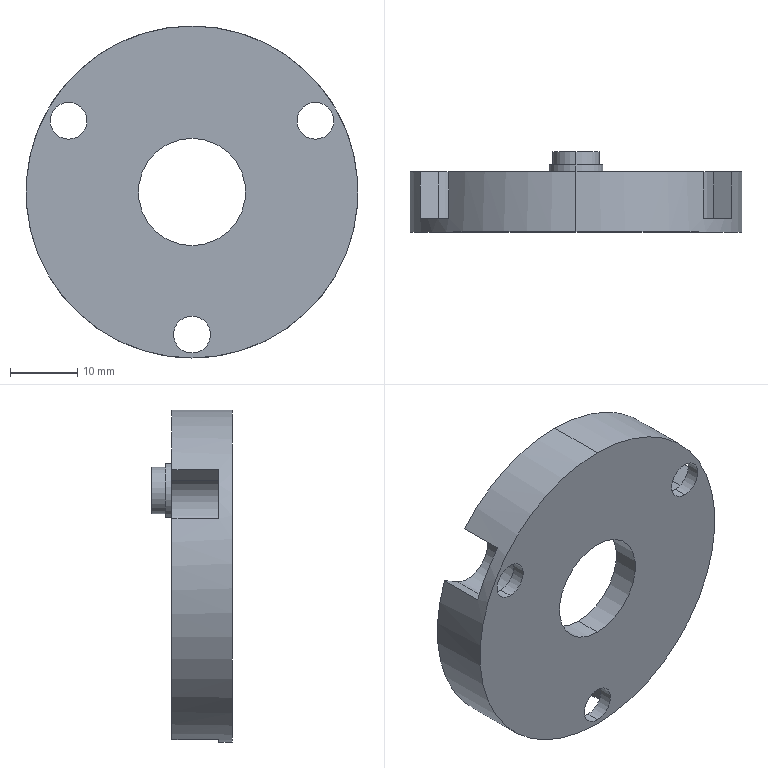Part | SolidWorks | features ICE 6, CirPattern 1, Extrusion 1, HoleWzd 1 | 1 solid | 44 faces | box 49.5 x 12 x 49.5 mm | volume 11403 mm3 | cylinder 26 | plane 14 | cone 4 | commonest cylinder face diameters 5.5 x6 4 x4 8.5 x4 5 x2 7 x2 8 x2
STEP:
#1=CARTESIAN_POINT('',(0.,4.,-8.));
#2=VERTEX_POINT('',#1);
#3=CARTESIAN_POINT('',(0.,4.,8.));
#4=VERTEX_POINT('',#3);
#5=CARTESIAN_POINT('',(0.,4.,0.));
#6=DIRECTION('',(0.,1.,0.));
#7=DIRECTION('',(0.,0.,1.));
#8=AXIS2_PLACEMENT_3D('',#5,#6,#7);
#9=CIRCLE('',#8,8.);
#10=EDGE_CURVE('',#2,#4,#9,.T.);
#11=ORIENTED_EDGE('',*,*,#10,.T.);
#12=CARTESIAN_POINT('',(0.,0.,8.));
#13=VERTEX_POINT('',#12);
#14=CARTESIAN_POINT('',(0.,5.,8.));
#15=DIRECTION('',(0.,-1.,0.));
#16=VECTOR('',#15,1000.);
#17=LINE('',#14,#16);
#18=EDGE_CURVE('',#4,#13,#17,.T.);
#19=ORIENTED_EDGE('',*,*,#18,.T.);
#20=CARTESIAN_POINT('',(0.,0.,-8.));
#21=VERTEX_POINT('',#20);
#22=CARTESIAN_POINT('',(0.,0.,0.));
#23=DIRECTION('',(0.,-1.,0.));
#24=DIRECTION('',(0.,0.,-1.));
#25=AXIS2_PLACEMENT_3D('',#22,#23,#24);
#26=CIRCLE('',#25,8.);
#27=EDGE_CURVE('',#13,#21,#26,.T.);
#28=ORIENTED_EDGE('',*,*,#27,.T.);
#29=CARTESIAN_POINT('',(0.,5.,-8.));
#30=DIRECTION('',(0.,-1.,0.));
#31=VECTOR('',#30,1000.);
#32=LINE('',#29,#31);
#33=EDGE_CURVE('',#2,#21,#32,.T.);
#34=ORIENTED_EDGE('',*,*,#33,.F.);
#35=EDGE_LOOP('',(#11,#19,#28,#34));
#36=FACE_OUTER_BOUND('',#35,.T.);
#37=CARTESIAN_POINT('',(0.,5.,0.));
#38=DIRECTION('',(0.,-1.,0.));
#39=DIRECTION('',(0.,0.,-1.));
#40=AXIS2_PLACEMENT_3D('',#37,#38,#39);
#41=CYLINDRICAL_SURFACE('',#40,8.);
#42=ADVANCED_FACE('',(#36),#41,.F.);
#43=CARTESIAN_POINT('',(9.28,4.,13.142));
#44=VERTEX_POINT('',#43);
#45=CARTESIAN_POINT('',(10.56,4.,12.678));
#46=VERTEX_POINT('',#45);
#47=CARTESIAN_POINT('',(9.28,4.,11.142));
#48=DIRECTION('',(0.,1.,0.));
#49=DIRECTION('',(0.,0.,1.));
#50=AXIS2_PLACEMENT_3D('',#47,#48,#49);
#51=CIRCLE('',#50,2.);
#52=EDGE_CURVE('',#44,#46,#51,.T.);
#53=ORIENTED_EDGE('',*,*,#52,.F.);
#54=CARTESIAN_POINT('',(9.28,9.,13.142));
#55=VERTEX_POINT('',#54);
#56=CARTESIAN_POINT('',(9.28,4.,13.142));
#57=DIRECTION('',(0.,1.,0.));
#58=VECTOR('',#57,1000.);
#59=LINE('',#56,#58);
#60=EDGE_CURVE('',#44,#55,#59,.T.);
#61=ORIENTED_EDGE('',*,*,#60,.T.);
#62=CARTESIAN_POINT('',(10.56,9.,12.678));
#63=VERTEX_POINT('',#62);
#64=CARTESIAN_POINT('',(9.28,9.,11.142));
#65=DIRECTION('',(0.,1.,0.));
#66=DIRECTION('',(0.,0.,1.));
#67=AXIS2_PLACEMENT_3D('',#64,#65,#66);
#68=CIRCLE('',#67,2.);
#69=EDGE_CURVE('',#55,#63,#68,.T.);
#70=ORIENTED_EDGE('',*,*,#69,.T.);
#71=CARTESIAN_POINT('',(10.56,4.,12.678));
#72=DIRECTION('',(0.,1.,0.));
#73=VECTOR('',#72,1000.);
#74=LINE('',#71,#73);
#75=EDGE_CURVE('',#46,#63,#74,.T.);
#76=ORIENTED_EDGE('',*,*,#75,.F.);
#77=EDGE_LOOP('',(#53,#61,#70,#76));
#78=FACE_OUTER_BOUND('',#77,.T.);
#79=CARTESIAN_POINT('',(9.28,4.,11.142));
#80=DIRECTION('',(0.,1.,0.));
#81=DIRECTION('',(0.,0.,1.));
#82=AXIS2_PLACEMENT_3D('',#79,#80,#81);
#83=CYLINDRICAL_SURFACE('',#82,2.);
#84=ADVANCED_FACE('',(#78),#83,.F.);
#85=CARTESIAN_POINT('',(-9.28,4.,13.142));
#86=VERTEX_POINT('',#85);
#87=CARTESIAN_POINT('',(-7.733,4.,12.41));
#88=VERTEX_POINT('',#87);
#89=CARTESIAN_POINT('',(-9.28,4.,11.142));
#90=DIRECTION('',(0.,1.,0.));
#91=DIRECTION('',(0.,0.,1.));
#92=AXIS2_PLACEMENT_3D('',#89,#90,#91);
#93=CIRCLE('',#92,2.);
#94=EDGE_CURVE('',#86,#88,#93,.T.);
#95=ORIENTED_EDGE('',*,*,#94,.F.);
#96=CARTESIAN_POINT('',(-9.28,9.,13.142));
#97=VERTEX_POINT('',#96);
#98=CARTESIAN_POINT('',(-9.28,4.,13.142));
#99=DIRECTION('',(0.,1.,0.));
#100=VECTOR('',#99,1000.);
#101=LINE('',#98,#100);
#102=EDGE_CURVE('',#86,#97,#101,.T.);
#103=ORIENTED_EDGE('',*,*,#102,.T.);
#104=CARTESIAN_POINT('',(-7.733,9.,12.41));
#105=VERTEX_POINT('',#104);
#106=CARTESIAN_POINT('',(-9.28,9.,11.142));
#107=DIRECTION('',(0.,1.,0.));
#108=DIRECTION('',(0.,0.,1.));
#109=AXIS2_PLACEMENT_3D('',#106,#107,#108);
#110=CIRCLE('',#109,2.);
#111=EDGE_CURVE('',#97,#105,#110,.T.);
#112=ORIENTED_EDGE('',*,*,#111,.T.);
#113=CARTESIAN_POINT('',(-7.733,4.,12.41));
#114=DIRECTION('',(0.,1.,0.));
#115=VECTOR('',#114,1000.);
#116=LINE('',#113,#115);
#117=EDGE_CURVE('',#88,#105,#116,.T.);
#118=ORIENTED_EDGE('',*,*,#117,.F.);
#119=EDGE_LOOP('',(#95,#103,#112,#118));
#120=FACE_OUTER_BOUND('',#119,.T.);
#121=CARTESIAN_POINT('',(-9.28,4.,11.142));
#122=DIRECTION('',(0.,1.,0.));
#123=DIRECTION('',(0.,0.,1.));
#124=AXIS2_PLACEMENT_3D('',#121,#122,#123);
#125=CYLINDRICAL_SURFACE('',#124,2.);
#126=ADVANCED_FACE('',(#120),#125,.F.);
#127=CARTESIAN_POINT('',(0.,11.975,10.25));
#128=VERTEX_POINT('',#127);
#129=CARTESIAN_POINT('',(0.,11.975,15.25));
#130=VERTEX_POINT('',#129);
#131=CARTESIAN_POINT('',(0.,11.975,12.75));
#132=DIRECTION('',(0.,1.,0.));
#133=DIRECTION('',(0.,0.,1.));
#134=AXIS2_PLACEMENT_3D('',#131,#132,#133);
#135=CIRCLE('',#134,2.5);
#136=EDGE_CURVE('',#128,#130,#135,.T.);
#137=ORIENTED_EDGE('',*,*,#136,.F.);
#138=CARTESIAN_POINT('',(0.,12.,10.225));
#139=VERTEX_POINT('',#138);
#140=CARTESIAN_POINT('',(0.,12.,10.225));
#141=DIRECTION('',(0.,0.7071,-0.7071));
#142=VECTOR('',#141,1000.);
#143=LINE('',#140,#142);
#144=EDGE_CURVE('',#128,#139,#143,.T.);
#145=ORIENTED_EDGE('',*,*,#144,.T.);
#146=CARTESIAN_POINT('',(0.,12.,15.275));
#147=VERTEX_POINT('',#146);
#148=CARTESIAN_POINT('',(0.,12.,12.75));
#149=DIRECTION('',(0.,1.,0.));
#150=DIRECTION('',(0.,0.,1.));
#151=AXIS2_PLACEMENT_3D('',#148,#149,#150);
#152=CIRCLE('',#151,2.525);
#153=EDGE_CURVE('',#139,#147,#152,.T.);
#154=ORIENTED_EDGE('',*,*,#153,.T.);
#155=CARTESIAN_POINT('',(0.,12.,15.275));
#156=DIRECTION('',(0.,0.7071,0.7071));
#157=VECTOR('',#156,1000.);
#158=LINE('',#155,#157);
#159=EDGE_CURVE('',#130,#147,#158,.T.);
#160=ORIENTED_EDGE('',*,*,#159,.F.);
#161=EDGE_LOOP('',(#137,#145,#154,#160));
#162=FACE_OUTER_BOUND('',#161,.T.);
#163=CARTESIAN_POINT('',(0.,12.,12.75));
#164=DIRECTION('',(0.,1.,0.));
#165=DIRECTION('',(0.,0.,1.));
#166=AXIS2_PLACEMENT_3D('',#163,#164,#165);
#167=CONICAL_SURFACE('',#166,2.525,0.7854);
#168=ADVANCED_FACE('',(#162),#167,.F.);
#169=CARTESIAN_POINT('',(0.,7.,10.25));
#170=VERTEX_POINT('',#169);
#171=CARTESIAN_POINT('',(0.,7.,15.25));
#172=VERTEX_POINT('',#171);
#173=CARTESIAN_POINT('',(0.,7.,12.75));
#174=DIRECTION('',(0.,1.,0.));
#175=DIRECTION('',(0.,0.,1.));
#176=AXIS2_PLACEMENT_3D('',#173,#174,#175);
#177=CIRCLE('',#176,2.5);
#178=EDGE_CURVE('',#170,#172,#177,.T.);
#179=ORIENTED_EDGE('',*,*,#178,.F.);
#180=CARTESIAN_POINT('',(0.,12.,10.25));
#181=DIRECTION('',(0.,1.,0.));
#182=VECTOR('',#181,1000.);
#183=LINE('',#180,#182);
#184=EDGE_CURVE('',#170,#128,#183,.T.);
#185=ORIENTED_EDGE('',*,*,#184,.T.);
#186=ORIENTED_EDGE('',*,*,#136,.T.);
#187=CARTESIAN_POINT('',(0.,12.,15.25));
#188=DIRECTION('',(0.,1.,0.));
#189=VECTOR('',#188,1000.);
#190=LINE('',#187,#189);
#191=EDGE_CURVE('',#172,#130,#190,.T.);
#192=ORIENTED_EDGE('',*,*,#191,.F.);
#193=EDGE_LOOP('',(#179,#185,#186,#192));
#194=FACE_OUTER_BOUND('',#193,.T.);
#195=CARTESIAN_POINT('',(0.,12.,12.75));
#196=DIRECTION('',(0.,1.,0.));
#197=DIRECTION('',(0.,0.,1.));
#198=AXIS2_PLACEMENT_3D('',#195,#196,#197);
#199=CYLINDRICAL_SURFACE('',#198,2.5);
#200=ADVANCED_FACE('',(#194),#199,.F.);
#201=CARTESIAN_POINT('',(0.,5.498,12.75));
#202=VERTEX_POINT('',#201);
#203=CARTESIAN_POINT('',(0.,7.,15.25));
#204=DIRECTION('',(0.,0.515,0.8572));
#205=VECTOR('',#204,1000.);
#206=LINE('',#203,#205);
#207=EDGE_CURVE('',#202,#172,#206,.T.);
#208=ORIENTED_EDGE('',*,*,#207,.F.);
#209=CARTESIAN_POINT('',(0.,7.,10.25));
#210=DIRECTION('',(0.,0.515,-0.8572));
#211=VECTOR('',#210,1000.);
#212=LINE('',#209,#211);
#213=EDGE_CURVE('',#202,#170,#212,.T.);
#214=ORIENTED_EDGE('',*,*,#213,.T.);
#215=ORIENTED_EDGE('',*,*,#178,.T.);
#216=EDGE_LOOP('',(#208,#214,#215));
#217=FACE_OUTER_BOUND('',#216,.T.);
#218=CARTESIAN_POINT('',(0.,7.,12.75));
#219=DIRECTION('',(0.,1.,0.));
#220=DIRECTION('',(0.,0.,1.));
#221=AXIS2_PLACEMENT_3D('',#218,#219,#220);
#222=CONICAL_SURFACE('',#221,2.5,1.03);
#223=ADVANCED_FACE('',(#217),#222,.F.);
#224=CARTESIAN_POINT('',(0.,12.,16.25));
#225=VERTEX_POINT('',#224);
#226=CARTESIAN_POINT('',(0.,12.,9.25));
#227=VERTEX_POINT('',#226);
#228=CARTESIAN_POINT('',(0.,12.,12.75));
#229=DIRECTION('',(0.,1.,0.));
#230=DIRECTION('',(0.,0.,1.));
#231=AXIS2_PLACEMENT_3D('',#228,#229,#230);
#232=CIRCLE('',#231,3.5);
#233=EDGE_CURVE('',#225,#227,#232,.T.);
#234=ORIENTED_EDGE('',*,*,#233,.F.);
#235=CARTESIAN_POINT('',(0.,10.,16.25));
#236=VERTEX_POINT('',#235);
#237=CARTESIAN_POINT('',(0.,12.,16.25));
#238=DIRECTION('',(0.,-1.,0.));
#239=VECTOR('',#238,1000.);
#240=LINE('',#237,#239);
#241=EDGE_CURVE('',#225,#236,#240,.T.);
#242=ORIENTED_EDGE('',*,*,#241,.T.);
#243=CARTESIAN_POINT('',(0.,10.,9.25));
#244=VERTEX_POINT('',#243);
#245=CARTESIAN_POINT('',(0.,10.,12.75));
#246=DIRECTION('',(0.,-1.,0.));
#247=DIRECTION('',(0.,0.,1.));
#248=AXIS2_PLACEMENT_3D('',#245,#246,#247);
#249=CIRCLE('',#248,3.5);
#250=EDGE_CURVE('',#244,#236,#249,.T.);
#251=ORIENTED_EDGE('',*,*,#250,.F.);
#252=CARTESIAN_POINT('',(0.,12.,9.25));
#253=DIRECTION('',(0.,-1.,0.));
#254=VECTOR('',#253,1000.);
#255=LINE('',#252,#254);
#256=EDGE_CURVE('',#227,#244,#255,.T.);
#257=ORIENTED_EDGE('',*,*,#256,.F.);
#258=EDGE_LOOP('',(#234,#242,#251,#257));
#259=FACE_OUTER_BOUND('',#258,.T.);
#260=CARTESIAN_POINT('',(0.,12.,12.75));
#261=DIRECTION('',(0.,-1.,0.));
#262=DIRECTION('',(0.,0.,-1.));
#263=AXIS2_PLACEMENT_3D('',#260,#261,#262);
#264=CYLINDRICAL_SURFACE('',#263,3.5);
#265=ADVANCED_FACE('',(#259),#264,.T.);
#266=CARTESIAN_POINT('',(0.,10.,16.75));
#267=VERTEX_POINT('',#266);
#268=CARTESIAN_POINT('',(0.,10.,8.75));
#269=VERTEX_POINT('',#268);
#270=CARTESIAN_POINT('',(0.,10.,12.75));
#271=DIRECTION('',(0.,1.,0.));
#272=DIRECTION('',(0.,0.,1.));
#273=AXIS2_PLACEMENT_3D('',#270,#271,#272);
#274=CIRCLE('',#273,4.);
#275=EDGE_CURVE('',#267,#269,#274,.T.);
#276=ORIENTED_EDGE('',*,*,#275,.F.);
#277=CARTESIAN_POINT('',(0.,9.,16.75));
#278=VERTEX_POINT('',#277);
#279=CARTESIAN_POINT('',(0.,10.,16.75));
#280=DIRECTION('',(0.,-1.,0.));
#281=VECTOR('',#280,1000.);
#282=LINE('',#279,#281);
#283=EDGE_CURVE('',#267,#278,#282,.T.);
#284=ORIENTED_EDGE('',*,*,#283,.T.);
#285=CARTESIAN_POINT('',(0.,9.,8.75));
#286=VERTEX_POINT('',#285);
#287=CARTESIAN_POINT('',(0.,9.,12.75));
#288=DIRECTION('',(0.,1.,0.));
#289=DIRECTION('',(0.,0.,1.));
#290=AXIS2_PLACEMENT_3D('',#287,#288,#289);
#291=CIRCLE('',#290,4.);
#292=EDGE_CURVE('',#278,#286,#291,.T.);
#293=ORIENTED_EDGE('',*,*,#292,.T.);
#294=CARTESIAN_POINT('',(0.,10.,8.75));
#295=DIRECTION('',(0.,-1.,0.));
#296=VECTOR('',#295,1000.);
#297=LINE('',#294,#296);
#298=EDGE_CURVE('',#269,#286,#297,.T.);
#299=ORIENTED_EDGE('',*,*,#298,.F.);
#300=EDGE_LOOP('',(#276,#284,#293,#299));
#301=FACE_OUTER_BOUND('',#300,.T.);
#302=CARTESIAN_POINT('',(0.,10.,12.75));
#303=DIRECTION('',(0.,-1.,0.));
#304=DIRECTION('',(0.,0.,-1.));
#305=AXIS2_PLACEMENT_3D('',#302,#303,#304);
#306=CYLINDRICAL_SURFACE('',#305,4.);
#307=ADVANCED_FACE('',(#301),#306,.T.);
#308=CARTESIAN_POINT('',(18.403,0.,7.875));
#309=VERTEX_POINT('',#308);
#310=CARTESIAN_POINT('',(18.403,0.,13.375));
#311=VERTEX_POINT('',#310);
#312=CARTESIAN_POINT('',(18.403,0.,10.625));
#313=DIRECTION('',(0.,1.,0.));
#314=DIRECTION('',(0.,0.,1.));
#315=AXIS2_PLACEMENT_3D('',#312,#313,#314);
#316=CIRCLE('',#315,2.75);
#317=EDGE_CURVE('',#309,#311,#316,.T.);
#318=ORIENTED_EDGE('',*,*,#317,.F.);
#319=CARTESIAN_POINT('',(18.403,2.,7.875));
#320=VERTEX_POINT('',#319);
#321=CARTESIAN_POINT('',(18.403,-5.,7.875));
#322=DIRECTION('',(0.,1.,0.));
#323=VECTOR('',#322,1000.);
#324=LINE('',#321,#323);
#325=EDGE_CURVE('',#309,#320,#324,.T.);
#326=ORIENTED_EDGE('',*,*,#325,.T.);
#327=CARTESIAN_POINT('',(18.403,2.,13.375));
#328=VERTEX_POINT('',#327);
#329=CARTESIAN_POINT('',(18.403,2.,10.625));
#330=DIRECTION('',(0.,1.,0.));
#331=DIRECTION('',(-0.866,0.,-0.5));
#332=AXIS2_PLACEMENT_3D('',#329,#330,#331);
#333=CIRCLE('',#332,2.75);
#334=EDGE_CURVE('',#320,#328,#333,.T.);
#335=ORIENTED_EDGE('',*,*,#334,.T.);
#336=CARTESIAN_POINT('',(18.403,-5.,13.375));
#337=DIRECTION('',(0.,1.,0.));
#338=VECTOR('',#337,1000.);
#339=LINE('',#336,#338);
#340=EDGE_CURVE('',#311,#328,#339,.T.);
#341=ORIENTED_EDGE('',*,*,#340,.F.);
#342=EDGE_LOOP('',(#318,#326,#335,#341));
#343=FACE_OUTER_BOUND('',#342,.T.);
#344=CARTESIAN_POINT('',(18.403,-5.,10.625));
#345=DIRECTION('',(0.,1.,0.));
#346=DIRECTION('',(0.,0.,1.));
#347=AXIS2_PLACEMENT_3D('',#344,#345,#346);
#348=CYLINDRICAL_SURFACE('',#347,2.75);
#349=ADVANCED_FACE('',(#343),#348,.F.);
#350=CARTESIAN_POINT('',(-18.403,0.,7.875));
#351=VERTEX_POINT('',#350);
#352=CARTESIAN_POINT('',(-18.403,0.,13.375));
#353=VERTEX_POINT('',#352);
#354=CARTESIAN_POINT('',(-18.403,0.,10.625));
#355=DIRECTION('',(0.,1.,0.));
#356=DIRECTION('',(0.,0.,1.));
#357=AXIS2_PLACEMENT_3D('',#354,#355,#356);
#358=CIRCLE('',#357,2.75);
#359=EDGE_CURVE('',#351,#353,#358,.T.);
#360=ORIENTED_EDGE('',*,*,#359,.F.);
#361=CARTESIAN_POINT('',(-18.403,2.,7.875));
#362=VERTEX_POINT('',#361);
#363=CARTESIAN_POINT('',(-18.403,-5.,7.875));
#364=DIRECTION('',(0.,1.,0.));
#365=VECTOR('',#364,1000.);
#366=LINE('',#363,#365);
#367=EDGE_CURVE('',#351,#362,#366,.T.);
#368=ORIENTED_EDGE('',*,*,#367,.T.);
#369=CARTESIAN_POINT('',(-18.403,2.,13.375));
#370=VERTEX_POINT('',#369);
#371=CARTESIAN_POINT('',(-18.403,2.,10.625));
#372=DIRECTION('',(0.,1.,0.));
#373=DIRECTION('',(0.866,0.,-0.5));
#374=AXIS2_PLACEMENT_3D('',#371,#372,#373);
#375=CIRCLE('',#374,2.75);
#376=EDGE_CURVE('',#362,#370,#375,.T.);
#377=ORIENTED_EDGE('',*,*,#376,.T.);
#378=CARTESIAN_POINT('',(-18.403,-5.,13.375));
#379=DIRECTION('',(0.,1.,0.));
#380=VECTOR('',#379,1000.);
#381=LINE('',#378,#380);
#382=EDGE_CURVE('',#353,#370,#381,.T.);
#383=ORIENTED_EDGE('',*,*,#382,.F.);
#384=EDGE_LOOP('',(#360,#368,#377,#383));
#385=FACE_OUTER_BOUND('',#384,.T.);
#386=CARTESIAN_POINT('',(-18.403,-5.,10.625));
#387=DIRECTION('',(0.,1.,0.));
#388=DIRECTION('',(0.,0.,1.));
#389=AXIS2_PLACEMENT_3D('',#386,#387,#388);
#390=CYLINDRICAL_SURFACE('',#389,2.75);
#391=ADVANCED_FACE('',(#385),#390,.F.);
#392=CARTESIAN_POINT('',(0.,0.,-24.));
#393=VERTEX_POINT('',#392);
#394=CARTESIAN_POINT('',(0.,0.,-18.5));
#395=VERTEX_POINT('',#394);
#396=CARTESIAN_POINT('',(0.,0.,-21.25));
#397=DIRECTION('',(0.,1.,0.));
#398=DIRECTION('',(0.,0.,1.));
#399=AXIS2_PLACEMENT_3D('',#396,#397,#398);
#400=CIRCLE('',#399,2.75);
#401=EDGE_CURVE('',#393,#395,#400,.T.);
#402=ORIENTED_EDGE('',*,*,#401,.F.);
#403=CARTESIAN_POINT('',(0.,2.,-24.));
#404=VERTEX_POINT('',#403);
#405=CARTESIAN_POINT('',(0.,-5.,-24.));
#406=DIRECTION('',(0.,1.,0.));
#407=VECTOR('',#406,1000.);
#408=LINE('',#405,#407);
#409=EDGE_CURVE('',#393,#404,#408,.T.);
#410=ORIENTED_EDGE('',*,*,#409,.T.);
#411=CARTESIAN_POINT('',(0.,2.,-18.5));
#412=VERTEX_POINT('',#411);
#413=CARTESIAN_POINT('',(0.,2.,-21.25));
#414=DIRECTION('',(0.,1.,0.));
#415=DIRECTION('',(0.,0.,1.));
#416=AXIS2_PLACEMENT_3D('',#413,#414,#415);
#417=CIRCLE('',#416,2.75);
#418=EDGE_CURVE('',#404,#412,#417,.T.);
#419=ORIENTED_EDGE('',*,*,#418,.T.);
#420=CARTESIAN_POINT('',(0.,-5.,-18.5));
#421=DIRECTION('',(0.,1.,0.));
#422=VECTOR('',#421,1000.);
#423=LINE('',#420,#422);
#424=EDGE_CURVE('',#395,#412,#423,.T.);
#425=ORIENTED_EDGE('',*,*,#424,.F.);
#426=EDGE_LOOP('',(#402,#410,#419,#425));
#427=FACE_OUTER_BOUND('',#426,.T.);
#428=CARTESIAN_POINT('',(0.,-5.,-21.25));
#429=DIRECTION('',(0.,1.,0.));
#430=DIRECTION('',(0.,0.,1.));
#431=AXIS2_PLACEMENT_3D('',#428,#429,#430);
#432=CYLINDRICAL_SURFACE('',#431,2.75);
#433=ADVANCED_FACE('',(#427),#432,.F.);
#434=CARTESIAN_POINT('',(0.,2.,-17.));
#435=VERTEX_POINT('',#434);
#436=CARTESIAN_POINT('',(4.25,2.,-21.25));
#437=VERTEX_POINT('',#436);
#438=CARTESIAN_POINT('',(0.,2.,-21.25));
#439=DIRECTION('',(0.,1.,0.));
#440=DIRECTION('',(0.,0.,1.));
#441=AXIS2_PLACEMENT_3D('',#438,#439,#440);
#442=CIRCLE('',#441,4.25);
#443=EDGE_CURVE('',#435,#437,#442,.T.);
#444=ORIENTED_EDGE('',*,*,#443,.F.);
#445=CARTESIAN_POINT('',(0.,9.,-17.));
#446=VERTEX_POINT('',#445);
#447=CARTESIAN_POINT('',(0.,2.,-17.));
#448=DIRECTION('',(0.,1.,0.));
#449=VECTOR('',#448,1000.);
#450=LINE('',#447,#449);
#451=EDGE_CURVE('',#435,#446,#450,.T.);
#452=ORIENTED_EDGE('',*,*,#451,.T.);
#453=CARTESIAN_POINT('',(4.25,9.,-21.25));
#454=VERTEX_POINT('',#453);
#455=CARTESIAN_POINT('',(0.,9.,-21.25));
#456=DIRECTION('',(0.,1.,0.));
#457=DIRECTION('',(0.,0.,1.));
#458=AXIS2_PLACEMENT_3D('',#455,#456,#457);
#459=CIRCLE('',#458,4.25);
#460=EDGE_CURVE('',#446,#454,#459,.T.);
#461=ORIENTED_EDGE('',*,*,#460,.T.);
#462=CARTESIAN_POINT('',(4.25,2.,-21.25));
#463=DIRECTION('',(0.,1.,0.));
#464=VECTOR('',#463,1000.);
#465=LINE('',#462,#464);
#466=EDGE_CURVE('',#437,#454,#465,.T.);
#467=ORIENTED_EDGE('',*,*,#466,.F.);
#468=EDGE_LOOP('',(#444,#452,#461,#467));
#469=FACE_OUTER_BOUND('',#468,.T.);
#470=CARTESIAN_POINT('',(0.,2.,-21.25));
#471=DIRECTION('',(0.,1.,0.));
#472=DIRECTION('',(0.,0.,1.));
#473=AXIS2_PLACEMENT_3D('',#470,#471,#472);
#474=CYLINDRICAL_SURFACE('',#473,4.25);
#475=ADVANCED_FACE('',(#469),#474,.F.);
#476=CARTESIAN_POINT('',(0.,9.,24.75));
#477=VERTEX_POINT('',#476);
#478=CARTESIAN_POINT('',(18.991,9.,15.872));
#479=VERTEX_POINT('',#478);
#480=CARTESIAN_POINT('',(0.,9.,0.));
#481=DIRECTION('',(0.,1.,0.));
#482=DIRECTION('',(0.,0.,1.));
#483=AXIS2_PLACEMENT_3D('',#480,#481,#482);
#484=CIRCLE('',#483,24.75);
#485=EDGE_CURVE('',#477,#479,#484,.T.);
#486=ORIENTED_EDGE('',*,*,#485,.F.);
#487=CARTESIAN_POINT('',(0.,0.,24.75));
#488=VERTEX_POINT('',#487);
#489=CARTESIAN_POINT('',(0.,9.,24.75));
#490=DIRECTION('',(0.,-1.,0.));
#491=VECTOR('',#490,1000.);
#492=LINE('',#489,#491);
#493=EDGE_CURVE('',#477,#488,#492,.T.);
#494=ORIENTED_EDGE('',*,*,#493,.T.);
#495=CARTESIAN_POINT('',(0.,0.,-24.75));
#496=VERTEX_POINT('',#495);
#497=CARTESIAN_POINT('',(0.,0.,0.));
#498=DIRECTION('',(0.,1.,0.));
#499=DIRECTION('',(0.,0.,1.));
#500=AXIS2_PLACEMENT_3D('',#497,#498,#499);
#501=CIRCLE('',#500,24.75);
#502=EDGE_CURVE('',#488,#496,#501,.T.);
#503=ORIENTED_EDGE('',*,*,#502,.T.);
#504=CARTESIAN_POINT('',(0.,2.,-24.75));
#505=VERTEX_POINT('',#504);
#506=CARTESIAN_POINT('',(0.,9.,-24.75));
#507=DIRECTION('',(0.,-1.,0.));
#508=VECTOR('',#507,1000.);
#509=LINE('',#506,#508);
#510=EDGE_CURVE('',#505,#496,#509,.T.);
#511=ORIENTED_EDGE('',*,*,#510,.F.);
#512=CARTESIAN_POINT('',(4.25,2.,-24.382));
#513=VERTEX_POINT('',#512);
#514=CARTESIAN_POINT('',(0.,2.,0.));
#515=DIRECTION('',(0.,1.,0.));
#516=DIRECTION('',(0.,0.,1.));
#517=AXIS2_PLACEMENT_3D('',#514,#515,#516);
#518=CIRCLE('',#517,24.75);
#519=EDGE_CURVE('',#513,#505,#518,.T.);
#520=ORIENTED_EDGE('',*,*,#519,.F.);
#521=CARTESIAN_POINT('',(4.25,9.,-24.382));
#522=VERTEX_POINT('',#521);
#523=CARTESIAN_POINT('',(4.25,9.,-24.382));
#524=DIRECTION('',(0.,-1.,0.));
#525=VECTOR('',#524,1000.);
#526=LINE('',#523,#525);
#527=EDGE_CURVE('',#522,#513,#526,.T.);
#528=ORIENTED_EDGE('',*,*,#527,.F.);
#529=CARTESIAN_POINT('',(23.241,9.,8.511));
#530=VERTEX_POINT('',#529);
#531=CARTESIAN_POINT('',(0.,9.,0.));
#532=DIRECTION('',(0.,1.,0.));
#533=DIRECTION('',(0.,0.,1.));
#534=AXIS2_PLACEMENT_3D('',#531,#532,#533);
#535=CIRCLE('',#534,24.75);
#536=EDGE_CURVE('',#530,#522,#535,.T.);
#537=ORIENTED_EDGE('',*,*,#536,.F.);
#538=CARTESIAN_POINT('',(23.241,2.,8.511));
#539=VERTEX_POINT('',#538);
#540=CARTESIAN_POINT('',(23.241,9.,8.511));
#541=DIRECTION('',(0.,1.,0.));
#542=VECTOR('',#541,1000.);
#543=LINE('',#540,#542);
#544=EDGE_CURVE('',#539,#530,#543,.T.);
#545=ORIENTED_EDGE('',*,*,#544,.F.);
#546=CARTESIAN_POINT('',(18.991,2.,15.872));
#547=VERTEX_POINT('',#546);
#548=CARTESIAN_POINT('',(0.,2.,0.));
#549=DIRECTION('',(0.,1.,0.));
#550=DIRECTION('',(0.,0.,1.));
#551=AXIS2_PLACEMENT_3D('',#548,#549,#550);
#552=CIRCLE('',#551,24.75);
#553=EDGE_CURVE('',#547,#539,#552,.T.);
#554=ORIENTED_EDGE('',*,*,#553,.F.);
#555=CARTESIAN_POINT('',(18.991,9.,15.872));
#556=DIRECTION('',(0.,-1.,0.));
#557=VECTOR('',#556,1000.);
#558=LINE('',#555,#557);
#559=EDGE_CURVE('',#479,#547,#558,.T.);
#560=ORIENTED_EDGE('',*,*,#559,.F.);
#561=EDGE_LOOP('',(#486,#494,#503,#511,#520,#528,#537,#545,#554,#560));
#562=FACE_OUTER_BOUND('',#561,.T.);
#563=CARTESIAN_POINT('',(0.,9.,0.));
#564=DIRECTION('',(0.,-1.,0.));
#565=DIRECTION('',(0.,0.,-1.));
#566=AXIS2_PLACEMENT_3D('',#563,#564,#565);
#567=CYLINDRICAL_SURFACE('',#566,24.75);
#568=ADVANCED_FACE('',(#562),#567,.T.);
#569=CARTESIAN_POINT('',(-4.25,9.,-24.382));
#570=VERTEX_POINT('',#569);
#571=CARTESIAN_POINT('',(-23.241,9.,8.511));
#572=VERTEX_POINT('',#571);
#573=CARTESIAN_POINT('',(0.,9.,0.));
#574=DIRECTION('',(0.,1.,0.));
#575=DIRECTION('',(0.,0.,1.));
#576=AXIS2_PLACEMENT_3D('',#573,#574,#575);
#577=CIRCLE('',#576,24.75);
#578=EDGE_CURVE('',#570,#572,#577,.T.);
#579=ORIENTED_EDGE('',*,*,#578,.T.);
#580=CARTESIAN_POINT('',(-20.528,9.,6.944));
#581=VERTEX_POINT('',#580);
#582=CARTESIAN_POINT('',(-2.125,9.,-3.681));
#583=DIRECTION('',(0.866,0.,-0.5));
#584=VECTOR('',#583,1000.);
#585=LINE('',#582,#584);
#586=EDGE_CURVE('',#572,#581,#585,.T.);
#587=ORIENTED_EDGE('',*,*,#586,.T.);
#588=CARTESIAN_POINT('',(-16.278,9.,14.306));
#589=VERTEX_POINT('',#588);
#590=CARTESIAN_POINT('',(-18.403,9.,10.625));
#591=DIRECTION('',(0.,1.,0.));
#592=DIRECTION('',(0.,0.,1.));
#593=AXIS2_PLACEMENT_3D('',#590,#591,#592);
#594=CIRCLE('',#593,4.25);
#595=EDGE_CURVE('',#589,#581,#594,.T.);
#596=ORIENTED_EDGE('',*,*,#595,.F.);
#597=CARTESIAN_POINT('',(-18.991,9.,15.872));
#598=VERTEX_POINT('',#597);
#599=CARTESIAN_POINT('',(2.125,9.,3.681));
#600=DIRECTION('',(-0.866,0.,0.5));
#601=VECTOR('',#600,1000.);
#602=LINE('',#599,#601);
#603=EDGE_CURVE('',#589,#598,#602,.T.);
#604=ORIENTED_EDGE('',*,*,#603,.T.);
#605=CARTESIAN_POINT('',(0.,9.,0.));
#606=DIRECTION('',(0.,1.,0.));
#607=DIRECTION('',(0.,0.,1.));
#608=AXIS2_PLACEMENT_3D('',#605,#606,#607);
#609=CIRCLE('',#608,24.75);
#610=EDGE_CURVE('',#598,#477,#609,.T.);
#611=ORIENTED_EDGE('',*,*,#610,.T.);
#612=ORIENTED_EDGE('',*,*,#485,.T.);
#613=CARTESIAN_POINT('',(16.278,9.,14.306));
#614=VERTEX_POINT('',#613);
#615=CARTESIAN_POINT('',(-2.125,9.,3.681));
#616=DIRECTION('',(-0.866,0.,-0.5));
#617=VECTOR('',#616,1000.);
#618=LINE('',#615,#617);
#619=EDGE_CURVE('',#479,#614,#618,.T.);
#620=ORIENTED_EDGE('',*,*,#619,.T.);
#621=CARTESIAN_POINT('',(20.528,9.,6.944));
#622=VERTEX_POINT('',#621);
#623=CARTESIAN_POINT('',(18.403,9.,10.625));
#624=DIRECTION('',(0.,1.,0.));
#625=DIRECTION('',(0.,0.,1.));
#626=AXIS2_PLACEMENT_3D('',#623,#624,#625);
#627=CIRCLE('',#626,4.25);
#628=EDGE_CURVE('',#622,#614,#627,.T.);
#629=ORIENTED_EDGE('',*,*,#628,.F.);
#630=CARTESIAN_POINT('',(2.125,9.,-3.681));
#631=DIRECTION('',(0.866,0.,0.5));
#632=VECTOR('',#631,1000.);
#633=LINE('',#630,#632);
#634=EDGE_CURVE('',#622,#530,#633,.T.);
#635=ORIENTED_EDGE('',*,*,#634,.T.);
#636=ORIENTED_EDGE('',*,*,#536,.T.);
#637=CARTESIAN_POINT('',(4.25,9.,0.));
#638=DIRECTION('',(0.,0.,1.));
#639=VECTOR('',#638,1000.);
#640=LINE('',#637,#639);
#641=EDGE_CURVE('',#522,#454,#640,.T.);
#642=ORIENTED_EDGE('',*,*,#641,.T.);
#643=ORIENTED_EDGE('',*,*,#460,.F.);
#644=CARTESIAN_POINT('',(-4.25,9.,-21.25));
#645=VERTEX_POINT('',#644);
#646=CARTESIAN_POINT('',(0.,9.,-21.25));
#647=DIRECTION('',(0.,1.,0.));
#648=DIRECTION('',(0.,0.,1.));
#649=AXIS2_PLACEMENT_3D('',#646,#647,#648);
#650=CIRCLE('',#649,4.25);
#651=EDGE_CURVE('',#645,#446,#650,.T.);
#652=ORIENTED_EDGE('',*,*,#651,.F.);
#653=CARTESIAN_POINT('',(-4.25,9.,0.));
#654=DIRECTION('',(0.,0.,-1.));
#655=VECTOR('',#654,1000.);
#656=LINE('',#653,#655);
#657=EDGE_CURVE('',#645,#570,#656,.T.);
#658=ORIENTED_EDGE('',*,*,#657,.T.);
#659=EDGE_LOOP('',(#579,#587,#596,#604,#611,#612,#620,#629,#635,#636,#642,#643,#652,#658));
#660=FACE_OUTER_BOUND('',#659,.T.);
#661=CARTESIAN_POINT('',(7.733,9.,12.41));
#662=VERTEX_POINT('',#661);
#663=CARTESIAN_POINT('',(9.28,9.,11.142));
#664=DIRECTION('',(0.,1.,0.));
#665=DIRECTION('',(0.,0.,1.));
#666=AXIS2_PLACEMENT_3D('',#663,#664,#665);
#667=CIRCLE('',#666,2.);
#668=EDGE_CURVE('',#662,#55,#667,.T.);
#669=ORIENTED_EDGE('',*,*,#668,.F.);
#670=CARTESIAN_POINT('',(0.,9.,18.75));
#671=DIRECTION('',(0.,1.,0.));
#672=DIRECTION('',(0.,0.,1.));
#673=AXIS2_PLACEMENT_3D('',#670,#671,#672);
#674=CIRCLE('',#673,10.);
#675=EDGE_CURVE('',#662,#286,#674,.T.);
#676=ORIENTED_EDGE('',*,*,#675,.T.);
#677=ORIENTED_EDGE('',*,*,#292,.F.);
#678=CARTESIAN_POINT('',(0.,9.,12.75));
#679=DIRECTION('',(0.,1.,0.));
#680=DIRECTION('',(0.,0.,1.));
#681=AXIS2_PLACEMENT_3D('',#678,#679,#680);
#682=CIRCLE('',#681,4.);
#683=EDGE_CURVE('',#286,#278,#682,.T.);
#684=ORIENTED_EDGE('',*,*,#683,.F.);
#685=CARTESIAN_POINT('',(0.,9.,18.75));
#686=DIRECTION('',(0.,1.,0.));
#687=DIRECTION('',(0.,0.,1.));
#688=AXIS2_PLACEMENT_3D('',#685,#686,#687);
#689=CIRCLE('',#688,10.);
#690=EDGE_CURVE('',#286,#105,#689,.T.);
#691=ORIENTED_EDGE('',*,*,#690,.T.);
#692=ORIENTED_EDGE('',*,*,#111,.F.);
#693=CARTESIAN_POINT('',(-10.56,9.,12.678));
#694=VERTEX_POINT('',#693);
#695=CARTESIAN_POINT('',(-9.28,9.,11.142));
#696=DIRECTION('',(0.,1.,0.));
#697=DIRECTION('',(0.,0.,1.));
#698=AXIS2_PLACEMENT_3D('',#695,#696,#697);
#699=CIRCLE('',#698,2.);
#700=EDGE_CURVE('',#694,#97,#699,.T.);
#701=ORIENTED_EDGE('',*,*,#700,.F.);
#702=CARTESIAN_POINT('',(0.,9.,0.));
#703=DIRECTION('',(0.,1.,0.));
#704=DIRECTION('',(0.,0.,1.));
#705=AXIS2_PLACEMENT_3D('',#702,#703,#704);
#706=CIRCLE('',#705,16.5);
#707=EDGE_CURVE('',#63,#694,#706,.T.);
#708=ORIENTED_EDGE('',*,*,#707,.F.);
#709=ORIENTED_EDGE('',*,*,#69,.F.);
#710=EDGE_LOOP('',(#669,#676,#677,#684,#691,#692,#701,#708,#709));
#711=FACE_BOUND('',#710,.T.);
#712=CARTESIAN_POINT('',(0.,9.,0.));
#713=DIRECTION('',(0.,1.,0.));
#714=DIRECTION('',(0.,0.,1.));
#715=AXIS2_PLACEMENT_3D('',#712,#713,#714);
#716=PLANE('',#715);
#717=ADVANCED_FACE('',(#660,#711),#716,.T.);
#718=ORIENTED_EDGE('',*,*,#493,.F.);
#719=ORIENTED_EDGE('',*,*,#610,.F.);
#720=CARTESIAN_POINT('',(-18.991,2.,15.872));
#721=VERTEX_POINT('',#720);
#722=CARTESIAN_POINT('',(-18.991,9.,15.872));
#723=DIRECTION('',(0.,1.,0.));
#724=VECTOR('',#723,1000.);
#725=LINE('',#722,#724);
#726=EDGE_CURVE('',#721,#598,#725,.T.);
#727=ORIENTED_EDGE('',*,*,#726,.F.);
#728=CARTESIAN_POINT('',(-23.241,2.,8.511));
#729=VERTEX_POINT('',#728);
#730=CARTESIAN_POINT('',(0.,2.,0.));
#731=DIRECTION('',(0.,1.,0.));
#732=DIRECTION('',(0.,0.,1.));
#733=AXIS2_PLACEMENT_3D('',#730,#731,#732);
#734=CIRCLE('',#733,24.75);
#735=EDGE_CURVE('',#729,#721,#734,.T.);
#736=ORIENTED_EDGE('',*,*,#735,.F.);
#737=CARTESIAN_POINT('',(-23.241,9.,8.511));
#738=DIRECTION('',(0.,-1.,0.));
#739=VECTOR('',#738,1000.);
#740=LINE('',#737,#739);
#741=EDGE_CURVE('',#572,#729,#740,.T.);
#742=ORIENTED_EDGE('',*,*,#741,.F.);
#743=ORIENTED_EDGE('',*,*,#578,.F.);
#744=CARTESIAN_POINT('',(-4.25,2.,-24.382));
#745=VERTEX_POINT('',#744);
#746=CARTESIAN_POINT('',(-4.25,9.,-24.382));
#747=DIRECTION('',(0.,1.,0.));
#748=VECTOR('',#747,1000.);
#749=LINE('',#746,#748);
#750=EDGE_CURVE('',#745,#570,#749,.T.);
#751=ORIENTED_EDGE('',*,*,#750,.F.);
#752=CARTESIAN_POINT('',(0.,2.,0.));
#753=DIRECTION('',(0.,1.,0.));
#754=DIRECTION('',(0.,0.,1.));
#755=AXIS2_PLACEMENT_3D('',#752,#753,#754);
#756=CIRCLE('',#755,24.75);
#757=EDGE_CURVE('',#505,#745,#756,.T.);
#758=ORIENTED_EDGE('',*,*,#757,.F.);
#759=ORIENTED_EDGE('',*,*,#510,.T.);
#760=CARTESIAN_POINT('',(0.,0.,0.));
#761=DIRECTION('',(0.,1.,0.));
#762=DIRECTION('',(0.,0.,1.));
#763=AXIS2_PLACEMENT_3D('',#760,#761,#762);
#764=CIRCLE('',#763,24.75);
#765=EDGE_CURVE('',#496,#488,#764,.T.);
#766=ORIENTED_EDGE('',*,*,#765,.T.);
#767=EDGE_LOOP('',(#718,#719,#727,#736,#742,#743,#751,#758,#759,#766));
#768=FACE_OUTER_BOUND('',#767,.T.);
#769=CARTESIAN_POINT('',(0.,9.,0.));
#770=DIRECTION('',(0.,-1.,0.));
#771=DIRECTION('',(0.,0.,-1.));
#772=AXIS2_PLACEMENT_3D('',#769,#770,#771);
#773=CYLINDRICAL_SURFACE('',#772,24.75);
#774=ADVANCED_FACE('',(#768),#773,.T.);
#775=CARTESIAN_POINT('',(0.,0.,0.));
#776=DIRECTION('',(0.,-1.,0.));
#777=DIRECTION('',(0.,0.,-1.));
#778=AXIS2_PLACEMENT_3D('',#775,#776,#777);
#779=CIRCLE('',#778,8.);
#780=EDGE_CURVE('',#21,#13,#779,.T.);
#781=ORIENTED_EDGE('',*,*,#780,.F.);
#782=ORIENTED_EDGE('',*,*,#27,.F.);
#783=EDGE_LOOP('',(#781,#782));
#784=FACE_BOUND('',#783,.T.);
#785=CARTESIAN_POINT('',(-18.403,0.,10.625));
#786=DIRECTION('',(0.,1.,0.));
#787=DIRECTION('',(0.,0.,1.));
#788=AXIS2_PLACEMENT_3D('',#785,#786,#787);
#789=CIRCLE('',#788,2.75);
#790=EDGE_CURVE('',#353,#351,#789,.T.);
#791=ORIENTED_EDGE('',*,*,#790,.T.);
#792=ORIENTED_EDGE('',*,*,#359,.T.);
#793=EDGE_LOOP('',(#791,#792));
#794=FACE_BOUND('',#793,.T.);
#795=CARTESIAN_POINT('',(18.403,0.,10.625));
#796=DIRECTION('',(0.,1.,0.));
#797=DIRECTION('',(0.,0.,1.));
#798=AXIS2_PLACEMENT_3D('',#795,#796,#797);
#799=CIRCLE('',#798,2.75);
#800=EDGE_CURVE('',#311,#309,#799,.T.);
#801=ORIENTED_EDGE('',*,*,#800,.T.);
#802=ORIENTED_EDGE('',*,*,#317,.T.);
#803=EDGE_LOOP('',(#801,#802));
#804=FACE_BOUND('',#803,.T.);
#805=CARTESIAN_POINT('',(0.,0.,-21.25));
#806=DIRECTION('',(0.,1.,0.));
#807=DIRECTION('',(0.,0.,1.));
#808=AXIS2_PLACEMENT_3D('',#805,#806,#807);
#809=CIRCLE('',#808,2.75);
#810=EDGE_CURVE('',#395,#393,#809,.T.);
#811=ORIENTED_EDGE('',*,*,#810,.T.);
#812=ORIENTED_EDGE('',*,*,#401,.T.);
#813=EDGE_LOOP('',(#811,#812));
#814=FACE_BOUND('',#813,.T.);
#815=ORIENTED_EDGE('',*,*,#765,.F.);
#816=ORIENTED_EDGE('',*,*,#502,.F.);
#817=EDGE_LOOP('',(#815,#816));
#818=FACE_OUTER_BOUND('',#817,.T.);
#819=CARTESIAN_POINT('',(0.,0.,0.));
#820=DIRECTION('',(0.,1.,0.));
#821=DIRECTION('',(0.,0.,1.));
#822=AXIS2_PLACEMENT_3D('',#819,#820,#821);
#823=PLANE('',#822);
#824=ADVANCED_FACE('',(#784,#794,#804,#814,#818),#823,.F.);
#825=CARTESIAN_POINT('',(0.,2.,-21.25));
#826=DIRECTION('',(0.,1.,0.));
#827=DIRECTION('',(0.,0.,1.));
#828=AXIS2_PLACEMENT_3D('',#825,#826,#827);
#829=CIRCLE('',#828,2.75);
#830=EDGE_CURVE('',#412,#404,#829,.T.);
#831=ORIENTED_EDGE('',*,*,#830,.F.);
#832=ORIENTED_EDGE('',*,*,#418,.F.);
#833=EDGE_LOOP('',(#831,#832));
#834=FACE_BOUND('',#833,.T.);
#835=ORIENTED_EDGE('',*,*,#519,.T.);
#836=ORIENTED_EDGE('',*,*,#757,.T.);
#837=CARTESIAN_POINT('',(-4.25,2.,-21.25));
#838=VERTEX_POINT('',#837);
#839=CARTESIAN_POINT('',(-4.25,2.,-21.25));
#840=DIRECTION('',(0.,0.,1.));
#841=VECTOR('',#840,1000.);
#842=LINE('',#839,#841);
#843=EDGE_CURVE('',#745,#838,#842,.T.);
#844=ORIENTED_EDGE('',*,*,#843,.T.);
#845=CARTESIAN_POINT('',(0.,2.,-21.25));
#846=DIRECTION('',(0.,1.,0.));
#847=DIRECTION('',(0.,0.,1.));
#848=AXIS2_PLACEMENT_3D('',#845,#846,#847);
#849=CIRCLE('',#848,4.25);
#850=EDGE_CURVE('',#838,#435,#849,.T.);
#851=ORIENTED_EDGE('',*,*,#850,.T.);
#852=ORIENTED_EDGE('',*,*,#443,.T.);
#853=CARTESIAN_POINT('',(4.25,2.,-27.92));
#854=DIRECTION('',(0.,0.,-1.));
#855=VECTOR('',#854,1000.);
#856=LINE('',#853,#855);
#857=EDGE_CURVE('',#437,#513,#856,.T.);
#858=ORIENTED_EDGE('',*,*,#857,.T.);
#859=EDGE_LOOP('',(#835,#836,#844,#851,#852,#858));
#860=FACE_OUTER_BOUND('',#859,.T.);
#861=CARTESIAN_POINT('',(0.,2.,-21.25));
#862=DIRECTION('',(0.,1.,0.));
#863=DIRECTION('',(0.,0.,1.));
#864=AXIS2_PLACEMENT_3D('',#861,#862,#863);
#865=PLANE('',#864);
#866=ADVANCED_FACE('',(#834,#860),#865,.T.);
#867=ORIENTED_EDGE('',*,*,#527,.T.);
#868=ORIENTED_EDGE('',*,*,#857,.F.);
#869=ORIENTED_EDGE('',*,*,#466,.T.);
#870=ORIENTED_EDGE('',*,*,#641,.F.);
#871=EDGE_LOOP('',(#867,#868,#869,#870));
#872=FACE_OUTER_BOUND('',#871,.T.);
#873=CARTESIAN_POINT('',(4.25,9.,-27.92));
#874=DIRECTION('',(-1.,0.,0.));
#875=DIRECTION('',(0.,0.,1.));
#876=AXIS2_PLACEMENT_3D('',#873,#874,#875);
#877=PLANE('',#876);
#878=ADVANCED_FACE('',(#872),#877,.T.);
#879=ORIENTED_EDGE('',*,*,#750,.T.);
#880=ORIENTED_EDGE('',*,*,#657,.F.);
#881=CARTESIAN_POINT('',(-4.25,2.,-21.25));
#882=DIRECTION('',(0.,1.,0.));
#883=VECTOR('',#882,1000.);
#884=LINE('',#881,#883);
#885=EDGE_CURVE('',#838,#645,#884,.T.);
#886=ORIENTED_EDGE('',*,*,#885,.F.);
#887=ORIENTED_EDGE('',*,*,#843,.F.);
#888=EDGE_LOOP('',(#879,#880,#886,#887));
#889=FACE_OUTER_BOUND('',#888,.T.);
#890=CARTESIAN_POINT('',(-4.25,9.,-21.25));
#891=DIRECTION('',(1.,0.,0.));
#892=DIRECTION('',(0.,0.,-1.));
#893=AXIS2_PLACEMENT_3D('',#890,#891,#892);
#894=PLANE('',#893);
#895=ADVANCED_FACE('',(#889),#894,.T.);
#896=ORIENTED_EDGE('',*,*,#451,.F.);
#897=ORIENTED_EDGE('',*,*,#850,.F.);
#898=ORIENTED_EDGE('',*,*,#885,.T.);
#899=ORIENTED_EDGE('',*,*,#651,.T.);
#900=EDGE_LOOP('',(#896,#897,#898,#899));
#901=FACE_OUTER_BOUND('',#900,.T.);
#902=CARTESIAN_POINT('',(0.,2.,-21.25));
#903=DIRECTION('',(0.,1.,0.));
#904=DIRECTION('',(0.,0.,1.));
#905=AXIS2_PLACEMENT_3D('',#902,#903,#904);
#906=CYLINDRICAL_SURFACE('',#905,4.25);
#907=ADVANCED_FACE('',(#901),#906,.F.);
#908=ORIENTED_EDGE('',*,*,#409,.F.);
#909=ORIENTED_EDGE('',*,*,#810,.F.);
#910=ORIENTED_EDGE('',*,*,#424,.T.);
#911=ORIENTED_EDGE('',*,*,#830,.T.);
#912=EDGE_LOOP('',(#908,#909,#910,#911));
#913=FACE_OUTER_BOUND('',#912,.T.);
#914=CARTESIAN_POINT('',(0.,-5.,-21.25));
#915=DIRECTION('',(0.,1.,0.));
#916=DIRECTION('',(0.,0.,1.));
#917=AXIS2_PLACEMENT_3D('',#914,#915,#916);
#918=CYLINDRICAL_SURFACE('',#917,2.75);
#919=ADVANCED_FACE('',(#913),#918,.F.);
#920=CARTESIAN_POINT('',(18.403,2.,10.625));
#921=DIRECTION('',(0.,1.,0.));
#922=DIRECTION('',(-0.866,0.,-0.5));
#923=AXIS2_PLACEMENT_3D('',#920,#921,#922);
#924=CIRCLE('',#923,2.75);
#925=EDGE_CURVE('',#328,#320,#924,.T.);
#926=ORIENTED_EDGE('',*,*,#925,.F.);
#927=ORIENTED_EDGE('',*,*,#334,.F.);
#928=EDGE_LOOP('',(#926,#927));
#929=FACE_BOUND('',#928,.T.);
#930=ORIENTED_EDGE('',*,*,#553,.T.);
#931=CARTESIAN_POINT('',(20.528,2.,6.944));
#932=VERTEX_POINT('',#931);
#933=CARTESIAN_POINT('',(20.528,2.,6.944));
#934=DIRECTION('',(-0.866,0.,-0.5));
#935=VECTOR('',#934,1000.);
#936=LINE('',#933,#935);
#937=EDGE_CURVE('',#539,#932,#936,.T.);
#938=ORIENTED_EDGE('',*,*,#937,.T.);
#939=CARTESIAN_POINT('',(16.278,2.,14.306));
#940=VERTEX_POINT('',#939);
#941=CARTESIAN_POINT('',(18.403,2.,10.625));
#942=DIRECTION('',(0.,1.,0.));
#943=DIRECTION('',(-0.866,0.,-0.5));
#944=AXIS2_PLACEMENT_3D('',#941,#942,#943);
#945=CIRCLE('',#944,4.25);
#946=EDGE_CURVE('',#932,#940,#945,.T.);
#947=ORIENTED_EDGE('',*,*,#946,.T.);
#948=CARTESIAN_POINT('',(22.055,2.,17.641));
#949=DIRECTION('',(0.866,0.,0.5));
#950=VECTOR('',#949,1000.);
#951=LINE('',#948,#950);
#952=EDGE_CURVE('',#940,#547,#951,.T.);
#953=ORIENTED_EDGE('',*,*,#952,.T.);
#954=EDGE_LOOP('',(#930,#938,#947,#953));
#955=FACE_OUTER_BOUND('',#954,.T.);
#956=CARTESIAN_POINT('',(18.403,2.,10.625));
#957=DIRECTION('',(0.,1.,0.));
#958=DIRECTION('',(-0.866,0.,-0.5));
#959=AXIS2_PLACEMENT_3D('',#956,#957,#958);
#960=PLANE('',#959);
#961=ADVANCED_FACE('',(#929,#955),#960,.T.);
#962=ORIENTED_EDGE('',*,*,#559,.T.);
#963=ORIENTED_EDGE('',*,*,#952,.F.);
#964=CARTESIAN_POINT('',(16.278,2.,14.306));
#965=DIRECTION('',(0.,1.,0.));
#966=VECTOR('',#965,1000.);
#967=LINE('',#964,#966);
#968=EDGE_CURVE('',#940,#614,#967,.T.);
#969=ORIENTED_EDGE('',*,*,#968,.T.);
#970=ORIENTED_EDGE('',*,*,#619,.F.);
#971=EDGE_LOOP('',(#962,#963,#969,#970));
#972=FACE_OUTER_BOUND('',#971,.T.);
#973=CARTESIAN_POINT('',(22.055,9.,17.641));
#974=DIRECTION('',(0.5,0.,-0.866));
#975=DIRECTION('',(-0.866,0.,-0.5));
#976=AXIS2_PLACEMENT_3D('',#973,#974,#975);
#977=PLANE('',#976);
#978=ADVANCED_FACE('',(#972),#977,.T.);
#979=ORIENTED_EDGE('',*,*,#544,.T.);
#980=ORIENTED_EDGE('',*,*,#634,.F.);
#981=CARTESIAN_POINT('',(20.528,2.,6.944));
#982=DIRECTION('',(0.,1.,0.));
#983=VECTOR('',#982,1000.);
#984=LINE('',#981,#983);
#985=EDGE_CURVE('',#932,#622,#984,.T.);
#986=ORIENTED_EDGE('',*,*,#985,.F.);
#987=ORIENTED_EDGE('',*,*,#937,.F.);
#988=EDGE_LOOP('',(#979,#980,#986,#987));
#989=FACE_OUTER_BOUND('',#988,.T.);
#990=CARTESIAN_POINT('',(20.528,9.,6.944));
#991=DIRECTION('',(-0.5,0.,0.866));
#992=DIRECTION('',(0.866,0.,0.5));
#993=AXIS2_PLACEMENT_3D('',#990,#991,#992);
#994=PLANE('',#993);
#995=ADVANCED_FACE('',(#989),#994,.T.);
#996=ORIENTED_EDGE('',*,*,#628,.T.);
#997=ORIENTED_EDGE('',*,*,#968,.F.);
#998=ORIENTED_EDGE('',*,*,#946,.F.);
#999=ORIENTED_EDGE('',*,*,#985,.T.);
#1000=EDGE_LOOP('',(#996,#997,#998,#999));
#1001=FACE_OUTER_BOUND('',#1000,.T.);
#1002=CARTESIAN_POINT('',(18.403,2.,10.625));
#1003=DIRECTION('',(0.,1.,0.));
#1004=DIRECTION('',(0.,0.,1.));
#1005=AXIS2_PLACEMENT_3D('',#1002,#1003,#1004);
#1006=CYLINDRICAL_SURFACE('',#1005,4.25);
#1007=ADVANCED_FACE('',(#1001),#1006,.F.);
#1008=CARTESIAN_POINT('',(-18.403,2.,10.625));
#1009=DIRECTION('',(0.,1.,0.));
#1010=DIRECTION('',(0.866,0.,-0.5));
#1011=AXIS2_PLACEMENT_3D('',#1008,#1009,#1010);
#1012=CIRCLE('',#1011,2.75);
#1013=EDGE_CURVE('',#370,#362,#1012,.T.);
#1014=ORIENTED_EDGE('',*,*,#1013,.F.);
#1015=ORIENTED_EDGE('',*,*,#376,.F.);
#1016=EDGE_LOOP('',(#1014,#1015));
#1017=FACE_BOUND('',#1016,.T.);
#1018=ORIENTED_EDGE('',*,*,#735,.T.);
#1019=CARTESIAN_POINT('',(-16.278,2.,14.306));
#1020=VERTEX_POINT('',#1019);
#1021=CARTESIAN_POINT('',(-16.278,2.,14.306));
#1022=DIRECTION('',(0.866,0.,-0.5));
#1023=VECTOR('',#1022,1000.);
#1024=LINE('',#1021,#1023);
#1025=EDGE_CURVE('',#721,#1020,#1024,.T.);
#1026=ORIENTED_EDGE('',*,*,#1025,.T.);
#1027=CARTESIAN_POINT('',(-20.528,2.,6.944));
#1028=VERTEX_POINT('',#1027);
#1029=CARTESIAN_POINT('',(-18.403,2.,10.625));
#1030=DIRECTION('',(0.,1.,0.));
#1031=DIRECTION('',(0.866,0.,-0.5));
#1032=AXIS2_PLACEMENT_3D('',#1029,#1030,#1031);
#1033=CIRCLE('',#1032,4.25);
#1034=EDGE_CURVE('',#1020,#1028,#1033,.T.);
#1035=ORIENTED_EDGE('',*,*,#1034,.T.);
#1036=CARTESIAN_POINT('',(-26.305,2.,10.28));
#1037=DIRECTION('',(-0.866,0.,0.5));
#1038=VECTOR('',#1037,1000.);
#1039=LINE('',#1036,#1038);
#1040=EDGE_CURVE('',#1028,#729,#1039,.T.);
#1041=ORIENTED_EDGE('',*,*,#1040,.T.);
#1042=EDGE_LOOP('',(#1018,#1026,#1035,#1041));
#1043=FACE_OUTER_BOUND('',#1042,.T.);
#1044=CARTESIAN_POINT('',(-18.403,2.,10.625));
#1045=DIRECTION('',(0.,1.,0.));
#1046=DIRECTION('',(0.866,0.,-0.5));
#1047=AXIS2_PLACEMENT_3D('',#1044,#1045,#1046);
#1048=PLANE('',#1047);
#1049=ADVANCED_FACE('',(#1017,#1043),#1048,.T.);
#1050=ORIENTED_EDGE('',*,*,#741,.T.);
#1051=ORIENTED_EDGE('',*,*,#1040,.F.);
#1052=CARTESIAN_POINT('',(-20.528,2.,6.944));
#1053=DIRECTION('',(0.,1.,0.));
#1054=VECTOR('',#1053,1000.);
#1055=LINE('',#1052,#1054);
#1056=EDGE_CURVE('',#1028,#581,#1055,.T.);
#1057=ORIENTED_EDGE('',*,*,#1056,.T.);
#1058=ORIENTED_EDGE('',*,*,#586,.F.);
#1059=EDGE_LOOP('',(#1050,#1051,#1057,#1058));
#1060=FACE_OUTER_BOUND('',#1059,.T.);
#1061=CARTESIAN_POINT('',(-26.305,9.,10.28));
#1062=DIRECTION('',(0.5,0.,0.866));
#1063=DIRECTION('',(0.866,0.,-0.5));
#1064=AXIS2_PLACEMENT_3D('',#1061,#1062,#1063);
#1065=PLANE('',#1064);
#1066=ADVANCED_FACE('',(#1060),#1065,.T.);
#1067=ORIENTED_EDGE('',*,*,#726,.T.);
#1068=ORIENTED_EDGE('',*,*,#603,.F.);
#1069=CARTESIAN_POINT('',(-16.278,2.,14.306));
#1070=DIRECTION('',(0.,1.,0.));
#1071=VECTOR('',#1070,1000.);
#1072=LINE('',#1069,#1071);
#1073=EDGE_CURVE('',#1020,#589,#1072,.T.);
#1074=ORIENTED_EDGE('',*,*,#1073,.F.);
#1075=ORIENTED_EDGE('',*,*,#1025,.F.);
#1076=EDGE_LOOP('',(#1067,#1068,#1074,#1075));
#1077=FACE_OUTER_BOUND('',#1076,.T.);
#1078=CARTESIAN_POINT('',(-16.278,9.,14.306));
#1079=DIRECTION('',(-0.5,0.,-0.866));
#1080=DIRECTION('',(-0.866,0.,0.5));
#1081=AXIS2_PLACEMENT_3D('',#1078,#1079,#1080);
#1082=PLANE('',#1081);
#1083=ADVANCED_FACE('',(#1077),#1082,.T.);
#1084=ORIENTED_EDGE('',*,*,#595,.T.);
#1085=ORIENTED_EDGE('',*,*,#1056,.F.);
#1086=ORIENTED_EDGE('',*,*,#1034,.F.);
#1087=ORIENTED_EDGE('',*,*,#1073,.T.);
#1088=EDGE_LOOP('',(#1084,#1085,#1086,#1087));
#1089=FACE_OUTER_BOUND('',#1088,.T.);
#1090=CARTESIAN_POINT('',(-18.403,2.,10.625));
#1091=DIRECTION('',(0.,1.,0.));
#1092=DIRECTION('',(0.,0.,1.));
#1093=AXIS2_PLACEMENT_3D('',#1090,#1091,#1092);
#1094=CYLINDRICAL_SURFACE('',#1093,4.25);
#1095=ADVANCED_FACE('',(#1089),#1094,.F.);
#1096=ORIENTED_EDGE('',*,*,#367,.F.);
#1097=ORIENTED_EDGE('',*,*,#790,.F.);
#1098=ORIENTED_EDGE('',*,*,#382,.T.);
#1099=ORIENTED_EDGE('',*,*,#1013,.T.);
#1100=EDGE_LOOP('',(#1096,#1097,#1098,#1099));
#1101=FACE_OUTER_BOUND('',#1100,.T.);
#1102=CARTESIAN_POINT('',(-18.403,-5.,10.625));
#1103=DIRECTION('',(0.,1.,0.));
#1104=DIRECTION('',(0.,0.,1.));
#1105=AXIS2_PLACEMENT_3D('',#1102,#1103,#1104);
#1106=CYLINDRICAL_SURFACE('',#1105,2.75);
#1107=ADVANCED_FACE('',(#1101),#1106,.F.);
#1108=ORIENTED_EDGE('',*,*,#325,.F.);
#1109=ORIENTED_EDGE('',*,*,#800,.F.);
#1110=ORIENTED_EDGE('',*,*,#340,.T.);
#1111=ORIENTED_EDGE('',*,*,#925,.T.);
#1112=EDGE_LOOP('',(#1108,#1109,#1110,#1111));
#1113=FACE_OUTER_BOUND('',#1112,.T.);
#1114=CARTESIAN_POINT('',(18.403,-5.,10.625));
#1115=DIRECTION('',(0.,1.,0.));
#1116=DIRECTION('',(0.,0.,1.));
#1117=AXIS2_PLACEMENT_3D('',#1114,#1115,#1116);
#1118=CYLINDRICAL_SURFACE('',#1117,2.75);
#1119=ADVANCED_FACE('',(#1113),#1118,.F.);
#1120=ORIENTED_EDGE('',*,*,#283,.F.);
#1121=CARTESIAN_POINT('',(0.,10.,12.75));
#1122=DIRECTION('',(0.,1.,0.));
#1123=DIRECTION('',(0.,0.,1.));
#1124=AXIS2_PLACEMENT_3D('',#1121,#1122,#1123);
#1125=CIRCLE('',#1124,4.);
#1126=EDGE_CURVE('',#269,#267,#1125,.T.);
#1127=ORIENTED_EDGE('',*,*,#1126,.F.);
#1128=ORIENTED_EDGE('',*,*,#298,.T.);
#1129=ORIENTED_EDGE('',*,*,#683,.T.);
#1130=EDGE_LOOP('',(#1120,#1127,#1128,#1129));
#1131=FACE_OUTER_BOUND('',#1130,.T.);
#1132=CARTESIAN_POINT('',(0.,10.,12.75));
#1133=DIRECTION('',(0.,-1.,0.));
#1134=DIRECTION('',(0.,0.,-1.));
#1135=AXIS2_PLACEMENT_3D('',#1132,#1133,#1134);
#1136=CYLINDRICAL_SURFACE('',#1135,4.);
#1137=ADVANCED_FACE('',(#1131),#1136,.T.);
#1138=ORIENTED_EDGE('',*,*,#250,.T.);
#1139=CARTESIAN_POINT('',(0.,10.,12.75));
#1140=DIRECTION('',(0.,-1.,0.));
#1141=DIRECTION('',(0.,0.,1.));
#1142=AXIS2_PLACEMENT_3D('',#1139,#1140,#1141);
#1143=CIRCLE('',#1142,3.5);
#1144=EDGE_CURVE('',#236,#244,#1143,.T.);
#1145=ORIENTED_EDGE('',*,*,#1144,.T.);
#1146=EDGE_LOOP('',(#1138,#1145));
#1147=FACE_BOUND('',#1146,.T.);
#1148=ORIENTED_EDGE('',*,*,#1126,.T.);
#1149=ORIENTED_EDGE('',*,*,#275,.T.);
#1150=EDGE_LOOP('',(#1148,#1149));
#1151=FACE_OUTER_BOUND('',#1150,.T.);
#1152=CARTESIAN_POINT('',(0.,10.,12.75));
#1153=DIRECTION('',(0.,1.,0.));
#1154=DIRECTION('',(0.,0.,1.));
#1155=AXIS2_PLACEMENT_3D('',#1152,#1153,#1154);
#1156=PLANE('',#1155);
#1157=ADVANCED_FACE('',(#1147,#1151),#1156,.T.);
#1158=ORIENTED_EDGE('',*,*,#241,.F.);
#1159=CARTESIAN_POINT('',(0.,12.,12.75));
#1160=DIRECTION('',(0.,1.,0.));
#1161=DIRECTION('',(0.,0.,1.));
#1162=AXIS2_PLACEMENT_3D('',#1159,#1160,#1161);
#1163=CIRCLE('',#1162,3.5);
#1164=EDGE_CURVE('',#227,#225,#1163,.T.);
#1165=ORIENTED_EDGE('',*,*,#1164,.F.);
#1166=ORIENTED_EDGE('',*,*,#256,.T.);
#1167=ORIENTED_EDGE('',*,*,#1144,.F.);
#1168=EDGE_LOOP('',(#1158,#1165,#1166,#1167));
#1169=FACE_OUTER_BOUND('',#1168,.T.);
#1170=CARTESIAN_POINT('',(0.,12.,12.75));
#1171=DIRECTION('',(0.,-1.,0.));
#1172=DIRECTION('',(0.,0.,-1.));
#1173=AXIS2_PLACEMENT_3D('',#1170,#1171,#1172);
#1174=CYLINDRICAL_SURFACE('',#1173,3.5);
#1175=ADVANCED_FACE('',(#1169),#1174,.T.);
#1176=CARTESIAN_POINT('',(0.,12.,12.75));
#1177=DIRECTION('',(0.,1.,0.));
#1178=DIRECTION('',(0.,0.,1.));
#1179=AXIS2_PLACEMENT_3D('',#1176,#1177,#1178);
#1180=CIRCLE('',#1179,2.525);
#1181=EDGE_CURVE('',#147,#139,#1180,.T.);
#1182=ORIENTED_EDGE('',*,*,#1181,.F.);
#1183=ORIENTED_EDGE('',*,*,#153,.F.);
#1184=EDGE_LOOP('',(#1182,#1183));
#1185=FACE_BOUND('',#1184,.T.);
#1186=ORIENTED_EDGE('',*,*,#1164,.T.);
#1187=ORIENTED_EDGE('',*,*,#233,.T.);
#1188=EDGE_LOOP('',(#1186,#1187));
#1189=FACE_OUTER_BOUND('',#1188,.T.);
#1190=CARTESIAN_POINT('',(0.,12.,12.75));
#1191=DIRECTION('',(0.,1.,0.));
#1192=DIRECTION('',(0.,0.,1.));
#1193=AXIS2_PLACEMENT_3D('',#1190,#1191,#1192);
#1194=PLANE('',#1193);
#1195=ADVANCED_FACE('',(#1185,#1189),#1194,.T.);
#1196=ORIENTED_EDGE('',*,*,#213,.F.);
#1197=ORIENTED_EDGE('',*,*,#207,.T.);
#1198=CARTESIAN_POINT('',(0.,7.,12.75));
#1199=DIRECTION('',(0.,1.,0.));
#1200=DIRECTION('',(0.,0.,1.));
#1201=AXIS2_PLACEMENT_3D('',#1198,#1199,#1200);
#1202=CIRCLE('',#1201,2.5);
#1203=EDGE_CURVE('',#172,#170,#1202,.T.);
#1204=ORIENTED_EDGE('',*,*,#1203,.T.);
#1205=EDGE_LOOP('',(#1196,#1197,#1204));
#1206=FACE_OUTER_BOUND('',#1205,.T.);
#1207=CARTESIAN_POINT('',(0.,7.,12.75));
#1208=DIRECTION('',(0.,1.,0.));
#1209=DIRECTION('',(0.,0.,1.));
#1210=AXIS2_PLACEMENT_3D('',#1207,#1208,#1209);
#1211=CONICAL_SURFACE('',#1210,2.5,1.03);
#1212=ADVANCED_FACE('',(#1206),#1211,.F.);
#1213=ORIENTED_EDGE('',*,*,#184,.F.);
#1214=ORIENTED_EDGE('',*,*,#1203,.F.);
#1215=ORIENTED_EDGE('',*,*,#191,.T.);
#1216=CARTESIAN_POINT('',(0.,11.975,12.75));
#1217=DIRECTION('',(0.,1.,0.));
#1218=DIRECTION('',(0.,0.,1.));
#1219=AXIS2_PLACEMENT_3D('',#1216,#1217,#1218);
#1220=CIRCLE('',#1219,2.5);
#1221=EDGE_CURVE('',#130,#128,#1220,.T.);
#1222=ORIENTED_EDGE('',*,*,#1221,.T.);
#1223=EDGE_LOOP('',(#1213,#1214,#1215,#1222));
#1224=FACE_OUTER_BOUND('',#1223,.T.);
#1225=CARTESIAN_POINT('',(0.,12.,12.75));
#1226=DIRECTION('',(0.,1.,0.));
#1227=DIRECTION('',(0.,0.,1.));
#1228=AXIS2_PLACEMENT_3D('',#1225,#1226,#1227);
#1229=CYLINDRICAL_SURFACE('',#1228,2.5);
#1230=ADVANCED_FACE('',(#1224),#1229,.F.);
#1231=ORIENTED_EDGE('',*,*,#144,.F.);
#1232=ORIENTED_EDGE('',*,*,#1221,.F.);
#1233=ORIENTED_EDGE('',*,*,#159,.T.);
#1234=ORIENTED_EDGE('',*,*,#1181,.T.);
#1235=EDGE_LOOP('',(#1231,#1232,#1233,#1234));
#1236=FACE_OUTER_BOUND('',#1235,.T.);
#1237=CARTESIAN_POINT('',(0.,12.,12.75));
#1238=DIRECTION('',(0.,1.,0.));
#1239=DIRECTION('',(0.,0.,1.));
#1240=AXIS2_PLACEMENT_3D('',#1237,#1238,#1239);
#1241=CONICAL_SURFACE('',#1240,2.525,0.7854);
#1242=ADVANCED_FACE('',(#1236),#1241,.F.);
#1243=ORIENTED_EDGE('',*,*,#675,.F.);
#1244=CARTESIAN_POINT('',(7.733,4.,12.41));
#1245=VERTEX_POINT('',#1244);
#1246=CARTESIAN_POINT('',(7.733,4.,12.41));
#1247=DIRECTION('',(0.,1.,0.));
#1248=VECTOR('',#1247,1000.);
#1249=LINE('',#1246,#1248);
#1250=EDGE_CURVE('',#1245,#662,#1249,.T.);
#1251=ORIENTED_EDGE('',*,*,#1250,.F.);
#1252=CARTESIAN_POINT('',(0.,4.,18.75));
#1253=DIRECTION('',(0.,1.,0.));
#1254=DIRECTION('',(0.,0.,1.));
#1255=AXIS2_PLACEMENT_3D('',#1252,#1253,#1254);
#1256=CIRCLE('',#1255,10.);
#1257=EDGE_CURVE('',#1245,#88,#1256,.T.);
#1258=ORIENTED_EDGE('',*,*,#1257,.T.);
#1259=ORIENTED_EDGE('',*,*,#117,.T.);
#1260=ORIENTED_EDGE('',*,*,#690,.F.);
#1261=EDGE_LOOP('',(#1243,#1251,#1258,#1259,#1260));
#1262=FACE_OUTER_BOUND('',#1261,.T.);
#1263=CARTESIAN_POINT('',(0.,4.,18.75));
#1264=DIRECTION('',(0.,1.,0.));
#1265=DIRECTION('',(0.,0.,1.));
#1266=AXIS2_PLACEMENT_3D('',#1263,#1264,#1265);
#1267=CYLINDRICAL_SURFACE('',#1266,10.);
#1268=ADVANCED_FACE('',(#1262),#1267,.T.);
#1269=ORIENTED_EDGE('',*,*,#102,.F.);
#1270=CARTESIAN_POINT('',(-10.56,4.,12.678));
#1271=VERTEX_POINT('',#1270);
#1272=CARTESIAN_POINT('',(-9.28,4.,11.142));
#1273=DIRECTION('',(0.,1.,0.));
#1274=DIRECTION('',(0.,0.,1.));
#1275=AXIS2_PLACEMENT_3D('',#1272,#1273,#1274);
#1276=CIRCLE('',#1275,2.);
#1277=EDGE_CURVE('',#1271,#86,#1276,.T.);
#1278=ORIENTED_EDGE('',*,*,#1277,.F.);
#1279=CARTESIAN_POINT('',(-10.56,4.,12.678));
#1280=DIRECTION('',(0.,1.,0.));
#1281=VECTOR('',#1280,1000.);
#1282=LINE('',#1279,#1281);
#1283=EDGE_CURVE('',#1271,#694,#1282,.T.);
#1284=ORIENTED_EDGE('',*,*,#1283,.T.);
#1285=ORIENTED_EDGE('',*,*,#700,.T.);
#1286=EDGE_LOOP('',(#1269,#1278,#1284,#1285));
#1287=FACE_OUTER_BOUND('',#1286,.T.);
#1288=CARTESIAN_POINT('',(-9.28,4.,11.142));
#1289=DIRECTION('',(0.,1.,0.));
#1290=DIRECTION('',(0.,0.,1.));
#1291=AXIS2_PLACEMENT_3D('',#1288,#1289,#1290);
#1292=CYLINDRICAL_SURFACE('',#1291,2.);
#1293=ADVANCED_FACE('',(#1287),#1292,.F.);
#1294=ORIENTED_EDGE('',*,*,#707,.T.);
#1295=ORIENTED_EDGE('',*,*,#1283,.F.);
#1296=CARTESIAN_POINT('',(0.,4.,0.));
#1297=DIRECTION('',(0.,1.,0.));
#1298=DIRECTION('',(0.,0.,1.));
#1299=AXIS2_PLACEMENT_3D('',#1296,#1297,#1298);
#1300=CIRCLE('',#1299,16.5);
#1301=EDGE_CURVE('',#46,#1271,#1300,.T.);
#1302=ORIENTED_EDGE('',*,*,#1301,.F.);
#1303=ORIENTED_EDGE('',*,*,#75,.T.);
#1304=EDGE_LOOP('',(#1294,#1295,#1302,#1303));
#1305=FACE_OUTER_BOUND('',#1304,.T.);
#1306=CARTESIAN_POINT('',(0.,4.,0.));
#1307=DIRECTION('',(0.,1.,0.));
#1308=DIRECTION('',(0.,0.,1.));
#1309=AXIS2_PLACEMENT_3D('',#1306,#1307,#1308);
#1310=CYLINDRICAL_SURFACE('',#1309,16.5);
#1311=ADVANCED_FACE('',(#1305),#1310,.F.);
#1312=ORIENTED_EDGE('',*,*,#60,.F.);
#1313=CARTESIAN_POINT('',(9.28,4.,11.142));
#1314=DIRECTION('',(0.,1.,0.));
#1315=DIRECTION('',(0.,0.,1.));
#1316=AXIS2_PLACEMENT_3D('',#1313,#1314,#1315);
#1317=CIRCLE('',#1316,2.);
#1318=EDGE_CURVE('',#1245,#44,#1317,.T.);
#1319=ORIENTED_EDGE('',*,*,#1318,.F.);
#1320=ORIENTED_EDGE('',*,*,#1250,.T.);
#1321=ORIENTED_EDGE('',*,*,#668,.T.);
#1322=EDGE_LOOP('',(#1312,#1319,#1320,#1321));
#1323=FACE_OUTER_BOUND('',#1322,.T.);
#1324=CARTESIAN_POINT('',(9.28,4.,11.142));
#1325=DIRECTION('',(0.,1.,0.));
#1326=DIRECTION('',(0.,0.,1.));
#1327=AXIS2_PLACEMENT_3D('',#1324,#1325,#1326);
#1328=CYLINDRICAL_SURFACE('',#1327,2.);
#1329=ADVANCED_FACE('',(#1323),#1328,.F.);
#1330=ORIENTED_EDGE('',*,*,#10,.F.);
#1331=CARTESIAN_POINT('',(0.,4.,0.));
#1332=DIRECTION('',(0.,1.,0.));
#1333=DIRECTION('',(0.,0.,1.));
#1334=AXIS2_PLACEMENT_3D('',#1331,#1332,#1333);
#1335=CIRCLE('',#1334,8.);
#1336=EDGE_CURVE('',#4,#2,#1335,.T.);
#1337=ORIENTED_EDGE('',*,*,#1336,.F.);
#1338=EDGE_LOOP('',(#1330,#1337));
#1339=FACE_BOUND('',#1338,.T.);
#1340=ORIENTED_EDGE('',*,*,#1257,.F.);
#1341=ORIENTED_EDGE('',*,*,#1318,.T.);
#1342=ORIENTED_EDGE('',*,*,#52,.T.);
#1343=ORIENTED_EDGE('',*,*,#1301,.T.);
#1344=ORIENTED_EDGE('',*,*,#1277,.T.);
#1345=ORIENTED_EDGE('',*,*,#94,.T.);
#1346=EDGE_LOOP('',(#1340,#1341,#1342,#1343,#1344,#1345));
#1347=FACE_OUTER_BOUND('',#1346,.T.);
#1348=CARTESIAN_POINT('',(-4.64,4.,14.946));
#1349=DIRECTION('',(0.,1.,0.));
#1350=DIRECTION('',(0.,0.,1.));
#1351=AXIS2_PLACEMENT_3D('',#1348,#1349,#1350);
#1352=PLANE('',#1351);
#1353=ADVANCED_FACE('',(#1339,#1347),#1352,.T.);
#1354=ORIENTED_EDGE('',*,*,#18,.F.);
#1355=ORIENTED_EDGE('',*,*,#1336,.T.);
#1356=ORIENTED_EDGE('',*,*,#33,.T.);
#1357=ORIENTED_EDGE('',*,*,#780,.T.);
#1358=EDGE_LOOP('',(#1354,#1355,#1356,#1357));
#1359=FACE_OUTER_BOUND('',#1358,.T.);
#1360=CARTESIAN_POINT('',(0.,5.,0.));
#1361=DIRECTION('',(0.,-1.,0.));
#1362=DIRECTION('',(0.,0.,-1.));
#1363=AXIS2_PLACEMENT_3D('',#1360,#1361,#1362);
#1364=CYLINDRICAL_SURFACE('',#1363,8.);
#1365=ADVANCED_FACE('',(#1359),#1364,.F.);
#1366=CLOSED_SHELL('',(#42,#84,#126,#168,#200,#223,#265,#307,#349,#391,#433,#475,#568,#717,#774,#824,#866,#878,#895,#907,#919,#961,#978,#995,#1007,#1049,#1066,#1083,#1095,#1107,#1119,#1137,#1157,#1175,#1195,#1212,#1230,#1242,#1268,#1293,#1311,#1329,#1353,#1365));
#1367=MANIFOLD_SOLID_BREP('',#1366);
#1368=CARTESIAN_POINT('',(0.,0.,0.));
#1369=DIRECTION('',(0.,0.,1.));
#1370=DIRECTION('',(1.,0.,0.));
#1371=AXIS2_PLACEMENT_3D('',#1368,#1369,#1370);
#1372=(LENGTH_UNIT()NAMED_UNIT(*)SI_UNIT(.MILLI.,.METRE.));
#1373=UNCERTAINTY_MEASURE_WITH_UNIT(LENGTH_MEASURE(0.00001),#1372,'','');
#1374=(NAMED_UNIT(*)PLANE_ANGLE_UNIT()SI_UNIT($,.RADIAN.));
#1375=(NAMED_UNIT(*)SI_UNIT($,.STERADIAN.)SOLID_ANGLE_UNIT());
#1376=(GEOMETRIC_REPRESENTATION_CONTEXT(3)GLOBAL_UNCERTAINTY_ASSIGNED_CONTEXT((#1373))GLOBAL_UNIT_ASSIGNED_CONTEXT((#1372,#1374,#1375))REPRESENTATION_CONTEXT('',''));
#1377=ADVANCED_BREP_SHAPE_REPRESENTATION('',(#1367,#1371),#1376);